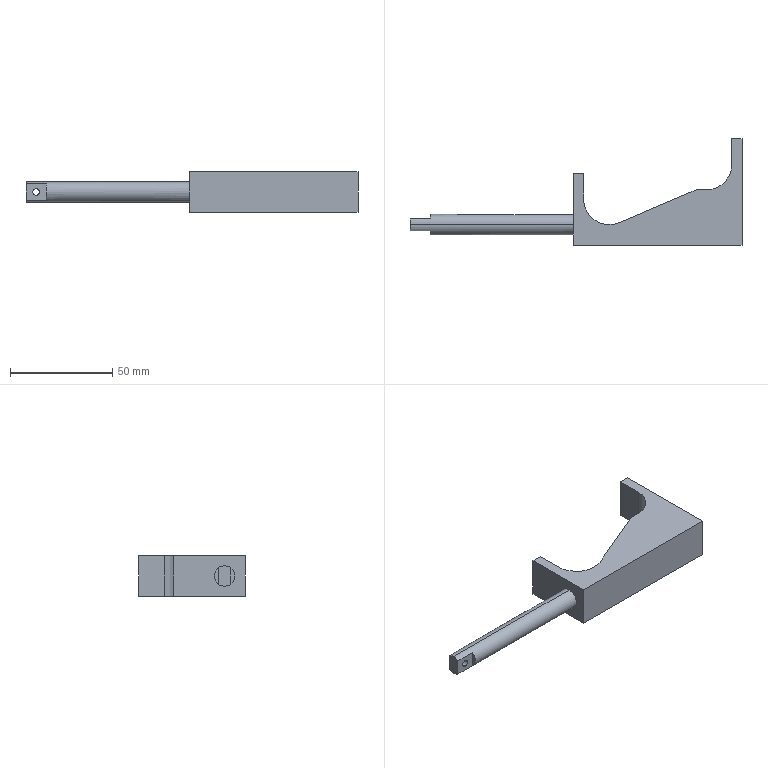Part | SolidWorks | features ICE 2, Extrusion 1, HoleWzd 1 | 1 solid | 22 faces | box 162.546 x 52 x 20 mm | volume 43317 mm3 | plane 16 | cylinder 6 | commonest cylinder face diameters 3.3 x2 10 x2 25 x2
STEP:
#1=CARTESIAN_POINT('',(-95.046,-3.,11.65));
#2=VERTEX_POINT('',#1);
#3=CARTESIAN_POINT('',(-95.046,-3.,8.35));
#4=VERTEX_POINT('',#3);
#5=CARTESIAN_POINT('',(-95.046,-3.,10.));
#6=DIRECTION('',(0.,-1.,0.));
#7=DIRECTION('',(0.,0.,-1.));
#8=AXIS2_PLACEMENT_3D('',#5,#6,#7);
#9=CIRCLE('',#8,1.65);
#10=EDGE_CURVE('',#2,#4,#9,.T.);
#11=ORIENTED_EDGE('',*,*,#10,.T.);
#12=CARTESIAN_POINT('',(-95.046,3.,8.35));
#13=VERTEX_POINT('',#12);
#14=CARTESIAN_POINT('',(-95.046,3.,8.35));
#15=DIRECTION('',(0.,1.,0.));
#16=VECTOR('',#15,1000.);
#17=LINE('',#14,#16);
#18=EDGE_CURVE('',#4,#13,#17,.T.);
#19=ORIENTED_EDGE('',*,*,#18,.T.);
#20=CARTESIAN_POINT('',(-95.046,3.,11.65));
#21=VERTEX_POINT('',#20);
#22=CARTESIAN_POINT('',(-95.046,3.,10.));
#23=DIRECTION('',(0.,1.,0.));
#24=DIRECTION('',(0.,0.,1.));
#25=AXIS2_PLACEMENT_3D('',#22,#23,#24);
#26=CIRCLE('',#25,1.65);
#27=EDGE_CURVE('',#13,#21,#26,.T.);
#28=ORIENTED_EDGE('',*,*,#27,.T.);
#29=CARTESIAN_POINT('',(-95.046,3.,11.65));
#30=DIRECTION('',(0.,1.,0.));
#31=VECTOR('',#30,1000.);
#32=LINE('',#29,#31);
#33=EDGE_CURVE('',#2,#21,#32,.T.);
#34=ORIENTED_EDGE('',*,*,#33,.F.);
#35=EDGE_LOOP('',(#11,#19,#28,#34));
#36=FACE_OUTER_BOUND('',#35,.T.);
#37=CARTESIAN_POINT('',(-95.046,3.,10.));
#38=DIRECTION('',(0.,1.,0.));
#39=DIRECTION('',(0.,0.,1.));
#40=AXIS2_PLACEMENT_3D('',#37,#38,#39);
#41=CYLINDRICAL_SURFACE('',#40,1.65);
#42=ADVANCED_FACE('',(#36),#41,.F.);
#43=CARTESIAN_POINT('',(-100.046,0.,15.));
#44=VERTEX_POINT('',#43);
#45=CARTESIAN_POINT('',(-100.046,3.,14.));
#46=VERTEX_POINT('',#45);
#47=CARTESIAN_POINT('',(-100.046,0.,10.));
#48=DIRECTION('',(-1.,0.,0.));
#49=DIRECTION('',(0.,0.,1.));
#50=AXIS2_PLACEMENT_3D('',#47,#48,#49);
#51=CIRCLE('',#50,5.);
#52=EDGE_CURVE('',#44,#46,#51,.T.);
#53=ORIENTED_EDGE('',*,*,#52,.F.);
#54=CARTESIAN_POINT('',(-20.046,0.,15.));
#55=VERTEX_POINT('',#54);
#56=CARTESIAN_POINT('',(-100.046,0.,15.));
#57=DIRECTION('',(1.,0.,0.));
#58=VECTOR('',#57,1000.);
#59=LINE('',#56,#58);
#60=EDGE_CURVE('',#44,#55,#59,.T.);
#61=ORIENTED_EDGE('',*,*,#60,.T.);
#62=CARTESIAN_POINT('',(-20.046,0.,5.));
#63=VERTEX_POINT('',#62);
#64=CARTESIAN_POINT('',(-20.046,0.,10.));
#65=DIRECTION('',(-1.,0.,0.));
#66=DIRECTION('',(0.,0.,-1.));
#67=AXIS2_PLACEMENT_3D('',#64,#65,#66);
#68=CIRCLE('',#67,5.);
#69=EDGE_CURVE('',#55,#63,#68,.T.);
#70=ORIENTED_EDGE('',*,*,#69,.T.);
#71=CARTESIAN_POINT('',(-100.046,0.,5.));
#72=VERTEX_POINT('',#71);
#73=CARTESIAN_POINT('',(-100.046,0.,5.));
#74=DIRECTION('',(1.,0.,0.));
#75=VECTOR('',#74,1000.);
#76=LINE('',#73,#75);
#77=EDGE_CURVE('',#72,#63,#76,.T.);
#78=ORIENTED_EDGE('',*,*,#77,.F.);
#79=CARTESIAN_POINT('',(-100.046,3.,6.));
#80=VERTEX_POINT('',#79);
#81=CARTESIAN_POINT('',(-100.046,0.,10.));
#82=DIRECTION('',(-1.,0.,0.));
#83=DIRECTION('',(0.,0.,1.));
#84=AXIS2_PLACEMENT_3D('',#81,#82,#83);
#85=CIRCLE('',#84,5.);
#86=EDGE_CURVE('',#80,#72,#85,.T.);
#87=ORIENTED_EDGE('',*,*,#86,.F.);
#88=CARTESIAN_POINT('',(-90.046,3.,6.));
#89=VERTEX_POINT('',#88);
#90=CARTESIAN_POINT('',(-100.046,3.,6.));
#91=DIRECTION('',(-1.,0.,0.));
#92=VECTOR('',#91,1000.);
#93=LINE('',#90,#92);
#94=EDGE_CURVE('',#89,#80,#93,.T.);
#95=ORIENTED_EDGE('',*,*,#94,.F.);
#96=CARTESIAN_POINT('',(-90.046,3.,14.));
#97=VERTEX_POINT('',#96);
#98=CARTESIAN_POINT('',(-90.046,0.,10.));
#99=DIRECTION('',(-1.,0.,0.));
#100=DIRECTION('',(0.,0.,1.));
#101=AXIS2_PLACEMENT_3D('',#98,#99,#100);
#102=CIRCLE('',#101,5.);
#103=EDGE_CURVE('',#97,#89,#102,.T.);
#104=ORIENTED_EDGE('',*,*,#103,.F.);
#105=CARTESIAN_POINT('',(-100.046,3.,14.));
#106=DIRECTION('',(1.,0.,0.));
#107=VECTOR('',#106,1000.);
#108=LINE('',#105,#107);
#109=EDGE_CURVE('',#46,#97,#108,.T.);
#110=ORIENTED_EDGE('',*,*,#109,.F.);
#111=EDGE_LOOP('',(#53,#61,#70,#78,#87,#95,#104,#110));
#112=FACE_OUTER_BOUND('',#111,.T.);
#113=CARTESIAN_POINT('',(-100.046,0.,10.));
#114=DIRECTION('',(1.,0.,0.));
#115=DIRECTION('',(0.,0.,-1.));
#116=AXIS2_PLACEMENT_3D('',#113,#114,#115);
#117=CYLINDRICAL_SURFACE('',#116,5.);
#118=ADVANCED_FACE('',(#112),#117,.T.);
#119=ORIENTED_EDGE('',*,*,#60,.F.);
#120=CARTESIAN_POINT('',(-100.046,-3.,14.));
#121=VERTEX_POINT('',#120);
#122=CARTESIAN_POINT('',(-100.046,0.,10.));
#123=DIRECTION('',(-1.,0.,0.));
#124=DIRECTION('',(0.,0.,1.));
#125=AXIS2_PLACEMENT_3D('',#122,#123,#124);
#126=CIRCLE('',#125,5.);
#127=EDGE_CURVE('',#121,#44,#126,.T.);
#128=ORIENTED_EDGE('',*,*,#127,.F.);
#129=CARTESIAN_POINT('',(-90.046,-3.,14.));
#130=VERTEX_POINT('',#129);
#131=CARTESIAN_POINT('',(-100.046,-3.,14.));
#132=DIRECTION('',(-1.,0.,0.));
#133=VECTOR('',#132,1000.);
#134=LINE('',#131,#133);
#135=EDGE_CURVE('',#130,#121,#134,.T.);
#136=ORIENTED_EDGE('',*,*,#135,.F.);
#137=CARTESIAN_POINT('',(-90.046,-3.,6.));
#138=VERTEX_POINT('',#137);
#139=CARTESIAN_POINT('',(-90.046,0.,10.));
#140=DIRECTION('',(-1.,0.,0.));
#141=DIRECTION('',(0.,0.,1.));
#142=AXIS2_PLACEMENT_3D('',#139,#140,#141);
#143=CIRCLE('',#142,5.);
#144=EDGE_CURVE('',#138,#130,#143,.T.);
#145=ORIENTED_EDGE('',*,*,#144,.F.);
#146=CARTESIAN_POINT('',(-100.046,-3.,6.));
#147=VERTEX_POINT('',#146);
#148=CARTESIAN_POINT('',(-100.046,-3.,6.));
#149=DIRECTION('',(1.,0.,0.));
#150=VECTOR('',#149,1000.);
#151=LINE('',#148,#150);
#152=EDGE_CURVE('',#147,#138,#151,.T.);
#153=ORIENTED_EDGE('',*,*,#152,.F.);
#154=CARTESIAN_POINT('',(-100.046,0.,10.));
#155=DIRECTION('',(-1.,0.,0.));
#156=DIRECTION('',(0.,0.,1.));
#157=AXIS2_PLACEMENT_3D('',#154,#155,#156);
#158=CIRCLE('',#157,5.);
#159=EDGE_CURVE('',#72,#147,#158,.T.);
#160=ORIENTED_EDGE('',*,*,#159,.F.);
#161=ORIENTED_EDGE('',*,*,#77,.T.);
#162=CARTESIAN_POINT('',(-20.046,0.,10.));
#163=DIRECTION('',(-1.,0.,0.));
#164=DIRECTION('',(0.,0.,-1.));
#165=AXIS2_PLACEMENT_3D('',#162,#163,#164);
#166=CIRCLE('',#165,5.);
#167=EDGE_CURVE('',#63,#55,#166,.T.);
#168=ORIENTED_EDGE('',*,*,#167,.T.);
#169=EDGE_LOOP('',(#119,#128,#136,#145,#153,#160,#161,#168));
#170=FACE_OUTER_BOUND('',#169,.T.);
#171=CARTESIAN_POINT('',(-100.046,0.,10.));
#172=DIRECTION('',(1.,0.,0.));
#173=DIRECTION('',(0.,0.,-1.));
#174=AXIS2_PLACEMENT_3D('',#171,#172,#173);
#175=CYLINDRICAL_SURFACE('',#174,5.);
#176=ADVANCED_FACE('',(#170),#175,.T.);
#177=ORIENTED_EDGE('',*,*,#127,.T.);
#178=ORIENTED_EDGE('',*,*,#52,.T.);
#179=CARTESIAN_POINT('',(-100.046,3.,10.));
#180=DIRECTION('',(0.,0.,-1.));
#181=VECTOR('',#180,1000.);
#182=LINE('',#179,#181);
#183=EDGE_CURVE('',#46,#80,#182,.T.);
#184=ORIENTED_EDGE('',*,*,#183,.T.);
#185=ORIENTED_EDGE('',*,*,#86,.T.);
#186=ORIENTED_EDGE('',*,*,#159,.T.);
#187=CARTESIAN_POINT('',(-100.046,-3.,10.));
#188=DIRECTION('',(0.,0.,1.));
#189=VECTOR('',#188,1000.);
#190=LINE('',#187,#189);
#191=EDGE_CURVE('',#147,#121,#190,.T.);
#192=ORIENTED_EDGE('',*,*,#191,.T.);
#193=EDGE_LOOP('',(#177,#178,#184,#185,#186,#192));
#194=FACE_OUTER_BOUND('',#193,.T.);
#195=CARTESIAN_POINT('',(-100.046,0.,10.));
#196=DIRECTION('',(-1.,0.,0.));
#197=DIRECTION('',(0.,0.,1.));
#198=AXIS2_PLACEMENT_3D('',#195,#196,#197);
#199=PLANE('',#198);
#200=ADVANCED_FACE('',(#194),#199,.T.);
#201=CARTESIAN_POINT('',(-20.046,25.,0.));
#202=VERTEX_POINT('',#201);
#203=CARTESIAN_POINT('',(-20.046,-10.,0.));
#204=VERTEX_POINT('',#203);
#205=CARTESIAN_POINT('',(-20.046,0.,0.));
#206=DIRECTION('',(0.,-1.,0.));
#207=VECTOR('',#206,1000.);
#208=LINE('',#205,#207);
#209=EDGE_CURVE('',#202,#204,#208,.T.);
#210=ORIENTED_EDGE('',*,*,#209,.T.);
#211=CARTESIAN_POINT('',(-20.046,-10.,20.));
#212=VERTEX_POINT('',#211);
#213=CARTESIAN_POINT('',(-20.046,-10.,20.));
#214=DIRECTION('',(0.,0.,-1.));
#215=VECTOR('',#214,1000.);
#216=LINE('',#213,#215);
#217=EDGE_CURVE('',#212,#204,#216,.T.);
#218=ORIENTED_EDGE('',*,*,#217,.F.);
#219=CARTESIAN_POINT('',(-20.046,25.,20.));
#220=VERTEX_POINT('',#219);
#221=CARTESIAN_POINT('',(-20.046,25.,20.));
#222=DIRECTION('',(0.,-1.,0.));
#223=VECTOR('',#222,1000.);
#224=LINE('',#221,#223);
#225=EDGE_CURVE('',#220,#212,#224,.T.);
#226=ORIENTED_EDGE('',*,*,#225,.F.);
#227=CARTESIAN_POINT('',(-20.046,25.,20.));
#228=DIRECTION('',(0.,0.,-1.));
#229=VECTOR('',#228,1000.);
#230=LINE('',#227,#229);
#231=EDGE_CURVE('',#220,#202,#230,.T.);
#232=ORIENTED_EDGE('',*,*,#231,.T.);
#233=EDGE_LOOP('',(#210,#218,#226,#232));
#234=FACE_OUTER_BOUND('',#233,.T.);
#235=ORIENTED_EDGE('',*,*,#167,.F.);
#236=ORIENTED_EDGE('',*,*,#69,.F.);
#237=EDGE_LOOP('',(#235,#236));
#238=FACE_BOUND('',#237,.T.);
#239=CARTESIAN_POINT('',(-20.046,0.,20.));
#240=DIRECTION('',(1.,0.,0.));
#241=DIRECTION('',(0.,0.,-1.));
#242=AXIS2_PLACEMENT_3D('',#239,#240,#241);
#243=PLANE('',#242);
#244=ADVANCED_FACE('',(#234,#238),#243,.F.);
#245=CARTESIAN_POINT('',(45.,17.,0.));
#246=VERTEX_POINT('',#245);
#247=CARTESIAN_POINT('',(40.,17.,0.));
#248=VERTEX_POINT('',#247);
#249=CARTESIAN_POINT('',(40.,17.,0.));
#250=DIRECTION('',(-1.,0.,0.));
#251=VECTOR('',#250,1000.);
#252=LINE('',#249,#251);
#253=EDGE_CURVE('',#246,#248,#252,.T.);
#254=ORIENTED_EDGE('',*,*,#253,.T.);
#255=CARTESIAN_POINT('',(40.,17.,20.));
#256=VERTEX_POINT('',#255);
#257=CARTESIAN_POINT('',(40.,17.,20.));
#258=DIRECTION('',(0.,0.,-1.));
#259=VECTOR('',#258,1000.);
#260=LINE('',#257,#259);
#261=EDGE_CURVE('',#256,#248,#260,.T.);
#262=ORIENTED_EDGE('',*,*,#261,.F.);
#263=CARTESIAN_POINT('',(45.,17.,20.));
#264=VERTEX_POINT('',#263);
#265=CARTESIAN_POINT('',(40.,17.,20.));
#266=DIRECTION('',(-1.,0.,0.));
#267=VECTOR('',#266,1000.);
#268=LINE('',#265,#267);
#269=EDGE_CURVE('',#264,#256,#268,.T.);
#270=ORIENTED_EDGE('',*,*,#269,.F.);
#271=CARTESIAN_POINT('',(45.,17.,20.));
#272=DIRECTION('',(0.,0.,-1.));
#273=VECTOR('',#272,1000.);
#274=LINE('',#271,#273);
#275=EDGE_CURVE('',#264,#246,#274,.T.);
#276=ORIENTED_EDGE('',*,*,#275,.T.);
#277=EDGE_LOOP('',(#254,#262,#270,#276));
#278=FACE_OUTER_BOUND('',#277,.T.);
#279=CARTESIAN_POINT('',(40.,17.,20.));
#280=DIRECTION('',(0.,-1.,0.));
#281=DIRECTION('',(1.,0.,0.));
#282=AXIS2_PLACEMENT_3D('',#279,#280,#281);
#283=PLANE('',#282);
#284=ADVANCED_FACE('',(#278),#283,.F.);
#285=CARTESIAN_POINT('',(2.343,0.9959,0.));
#286=VERTEX_POINT('',#285);
#287=CARTESIAN_POINT('',(2.343,0.9959,0.));
#288=DIRECTION('',(-0.9203,-0.3911,0.));
#289=VECTOR('',#288,1000.);
#290=LINE('',#287,#289);
#291=EDGE_CURVE('',#248,#286,#290,.T.);
#292=ORIENTED_EDGE('',*,*,#291,.T.);
#293=CARTESIAN_POINT('',(2.343,0.9959,20.));
#294=VERTEX_POINT('',#293);
#295=CARTESIAN_POINT('',(2.343,0.9959,20.));
#296=DIRECTION('',(0.,0.,-1.));
#297=VECTOR('',#296,1000.);
#298=LINE('',#295,#297);
#299=EDGE_CURVE('',#294,#286,#298,.T.);
#300=ORIENTED_EDGE('',*,*,#299,.F.);
#301=CARTESIAN_POINT('',(2.343,0.9959,20.));
#302=DIRECTION('',(-0.9203,-0.3911,0.));
#303=VECTOR('',#302,1000.);
#304=LINE('',#301,#303);
#305=EDGE_CURVE('',#256,#294,#304,.T.);
#306=ORIENTED_EDGE('',*,*,#305,.F.);
#307=ORIENTED_EDGE('',*,*,#261,.T.);
#308=EDGE_LOOP('',(#292,#300,#306,#307));
#309=FACE_OUTER_BOUND('',#308,.T.);
#310=CARTESIAN_POINT('',(2.343,0.9959,20.));
#311=DIRECTION('',(0.3911,-0.9203,0.));
#312=DIRECTION('',(0.9203,0.3911,0.));
#313=AXIS2_PLACEMENT_3D('',#310,#311,#312);
#314=PLANE('',#313);
#315=ADVANCED_FACE('',(#309),#314,.F.);
#316=CARTESIAN_POINT('',(-15.046,12.5,0.));
#317=VERTEX_POINT('',#316);
#318=CARTESIAN_POINT('',(-2.546,12.5,0.));
#319=DIRECTION('',(0.,0.,-1.));
#320=DIRECTION('',(1.,0.,0.));
#321=AXIS2_PLACEMENT_3D('',#318,#319,#320);
#322=CIRCLE('',#321,12.5);
#323=EDGE_CURVE('',#286,#317,#322,.T.);
#324=ORIENTED_EDGE('',*,*,#323,.T.);
#325=CARTESIAN_POINT('',(-15.046,12.5,20.));
#326=VERTEX_POINT('',#325);
#327=CARTESIAN_POINT('',(-15.046,12.5,20.));
#328=DIRECTION('',(0.,0.,-1.));
#329=VECTOR('',#328,1000.);
#330=LINE('',#327,#329);
#331=EDGE_CURVE('',#326,#317,#330,.T.);
#332=ORIENTED_EDGE('',*,*,#331,.F.);
#333=CARTESIAN_POINT('',(-2.546,12.5,20.));
#334=DIRECTION('',(0.,0.,-1.));
#335=DIRECTION('',(1.,0.,0.));
#336=AXIS2_PLACEMENT_3D('',#333,#334,#335);
#337=CIRCLE('',#336,12.5);
#338=EDGE_CURVE('',#294,#326,#337,.T.);
#339=ORIENTED_EDGE('',*,*,#338,.F.);
#340=ORIENTED_EDGE('',*,*,#299,.T.);
#341=EDGE_LOOP('',(#324,#332,#339,#340));
#342=FACE_OUTER_BOUND('',#341,.T.);
#343=CARTESIAN_POINT('',(-2.546,12.5,20.));
#344=DIRECTION('',(0.,0.,-1.));
#345=DIRECTION('',(-1.,0.,0.));
#346=AXIS2_PLACEMENT_3D('',#343,#344,#345);
#347=CYLINDRICAL_SURFACE('',#346,12.5);
#348=ADVANCED_FACE('',(#342),#347,.F.);
#349=CARTESIAN_POINT('',(-15.046,25.,0.));
#350=VERTEX_POINT('',#349);
#351=CARTESIAN_POINT('',(-15.046,12.5,0.));
#352=DIRECTION('',(0.,1.,0.));
#353=VECTOR('',#352,1000.);
#354=LINE('',#351,#353);
#355=EDGE_CURVE('',#317,#350,#354,.T.);
#356=ORIENTED_EDGE('',*,*,#355,.T.);
#357=CARTESIAN_POINT('',(-15.046,25.,20.));
#358=VERTEX_POINT('',#357);
#359=CARTESIAN_POINT('',(-15.046,25.,20.));
#360=DIRECTION('',(0.,0.,-1.));
#361=VECTOR('',#360,1000.);
#362=LINE('',#359,#361);
#363=EDGE_CURVE('',#358,#350,#362,.T.);
#364=ORIENTED_EDGE('',*,*,#363,.F.);
#365=CARTESIAN_POINT('',(-15.046,12.5,20.));
#366=DIRECTION('',(0.,1.,0.));
#367=VECTOR('',#366,1000.);
#368=LINE('',#365,#367);
#369=EDGE_CURVE('',#326,#358,#368,.T.);
#370=ORIENTED_EDGE('',*,*,#369,.F.);
#371=ORIENTED_EDGE('',*,*,#331,.T.);
#372=EDGE_LOOP('',(#356,#364,#370,#371));
#373=FACE_OUTER_BOUND('',#372,.T.);
#374=CARTESIAN_POINT('',(-15.046,12.5,20.));
#375=DIRECTION('',(-1.,0.,0.));
#376=DIRECTION('',(0.,0.,1.));
#377=AXIS2_PLACEMENT_3D('',#374,#375,#376);
#378=PLANE('',#377);
#379=ADVANCED_FACE('',(#373),#378,.F.);
#380=CARTESIAN_POINT('',(-15.046,25.,0.));
#381=DIRECTION('',(-1.,0.,0.));
#382=VECTOR('',#381,1000.);
#383=LINE('',#380,#382);
#384=EDGE_CURVE('',#350,#202,#383,.T.);
#385=ORIENTED_EDGE('',*,*,#384,.T.);
#386=ORIENTED_EDGE('',*,*,#231,.F.);
#387=CARTESIAN_POINT('',(-15.046,25.,20.));
#388=DIRECTION('',(-1.,0.,0.));
#389=VECTOR('',#388,1000.);
#390=LINE('',#387,#389);
#391=EDGE_CURVE('',#358,#220,#390,.T.);
#392=ORIENTED_EDGE('',*,*,#391,.F.);
#393=ORIENTED_EDGE('',*,*,#363,.T.);
#394=EDGE_LOOP('',(#385,#386,#392,#393));
#395=FACE_OUTER_BOUND('',#394,.T.);
#396=CARTESIAN_POINT('',(-15.046,25.,20.));
#397=DIRECTION('',(0.,-1.,0.));
#398=DIRECTION('',(0.,0.,-1.));
#399=AXIS2_PLACEMENT_3D('',#396,#397,#398);
#400=PLANE('',#399);
#401=ADVANCED_FACE('',(#395),#400,.F.);
#402=CARTESIAN_POINT('',(62.5,-10.,0.));
#403=VERTEX_POINT('',#402);
#404=CARTESIAN_POINT('',(57.5,-10.,0.));
#405=DIRECTION('',(1.,0.,0.));
#406=VECTOR('',#405,1000.);
#407=LINE('',#404,#406);
#408=EDGE_CURVE('',#204,#403,#407,.T.);
#409=ORIENTED_EDGE('',*,*,#408,.T.);
#410=CARTESIAN_POINT('',(62.5,-10.,20.));
#411=VERTEX_POINT('',#410);
#412=CARTESIAN_POINT('',(62.5,-10.,20.));
#413=DIRECTION('',(0.,0.,-1.));
#414=VECTOR('',#413,1000.);
#415=LINE('',#412,#414);
#416=EDGE_CURVE('',#411,#403,#415,.T.);
#417=ORIENTED_EDGE('',*,*,#416,.F.);
#418=CARTESIAN_POINT('',(-20.046,-10.,20.));
#419=DIRECTION('',(1.,0.,0.));
#420=VECTOR('',#419,1000.);
#421=LINE('',#418,#420);
#422=EDGE_CURVE('',#212,#411,#421,.T.);
#423=ORIENTED_EDGE('',*,*,#422,.F.);
#424=ORIENTED_EDGE('',*,*,#217,.T.);
#425=EDGE_LOOP('',(#409,#417,#423,#424));
#426=FACE_OUTER_BOUND('',#425,.T.);
#427=CARTESIAN_POINT('',(57.5,-10.,20.));
#428=DIRECTION('',(0.,1.,0.));
#429=DIRECTION('',(0.,0.,1.));
#430=AXIS2_PLACEMENT_3D('',#427,#428,#429);
#431=PLANE('',#430);
#432=ADVANCED_FACE('',(#426),#431,.F.);
#433=CARTESIAN_POINT('',(62.5,42.,0.));
#434=VERTEX_POINT('',#433);
#435=CARTESIAN_POINT('',(62.5,-10.,0.));
#436=DIRECTION('',(0.,1.,0.));
#437=VECTOR('',#436,1000.);
#438=LINE('',#435,#437);
#439=EDGE_CURVE('',#403,#434,#438,.T.);
#440=ORIENTED_EDGE('',*,*,#439,.T.);
#441=CARTESIAN_POINT('',(62.5,42.,20.));
#442=VERTEX_POINT('',#441);
#443=CARTESIAN_POINT('',(62.5,42.,20.));
#444=DIRECTION('',(0.,0.,-1.));
#445=VECTOR('',#444,1000.);
#446=LINE('',#443,#445);
#447=EDGE_CURVE('',#442,#434,#446,.T.);
#448=ORIENTED_EDGE('',*,*,#447,.F.);
#449=CARTESIAN_POINT('',(62.5,-10.,20.));
#450=DIRECTION('',(0.,1.,0.));
#451=VECTOR('',#450,1000.);
#452=LINE('',#449,#451);
#453=EDGE_CURVE('',#411,#442,#452,.T.);
#454=ORIENTED_EDGE('',*,*,#453,.F.);
#455=ORIENTED_EDGE('',*,*,#416,.T.);
#456=EDGE_LOOP('',(#440,#448,#454,#455));
#457=FACE_OUTER_BOUND('',#456,.T.);
#458=CARTESIAN_POINT('',(62.5,-10.,20.));
#459=DIRECTION('',(-1.,0.,0.));
#460=DIRECTION('',(0.,0.,1.));
#461=AXIS2_PLACEMENT_3D('',#458,#459,#460);
#462=PLANE('',#461);
#463=ADVANCED_FACE('',(#457),#462,.F.);
#464=CARTESIAN_POINT('',(57.5,42.,0.));
#465=VERTEX_POINT('',#464);
#466=CARTESIAN_POINT('',(62.5,42.,0.));
#467=DIRECTION('',(-1.,0.,0.));
#468=VECTOR('',#467,1000.);
#469=LINE('',#466,#468);
#470=EDGE_CURVE('',#434,#465,#469,.T.);
#471=ORIENTED_EDGE('',*,*,#470,.T.);
#472=CARTESIAN_POINT('',(57.5,42.,20.));
#473=VERTEX_POINT('',#472);
#474=CARTESIAN_POINT('',(57.5,42.,20.));
#475=DIRECTION('',(0.,0.,-1.));
#476=VECTOR('',#475,1000.);
#477=LINE('',#474,#476);
#478=EDGE_CURVE('',#473,#465,#477,.T.);
#479=ORIENTED_EDGE('',*,*,#478,.F.);
#480=CARTESIAN_POINT('',(62.5,42.,20.));
#481=DIRECTION('',(-1.,0.,0.));
#482=VECTOR('',#481,1000.);
#483=LINE('',#480,#482);
#484=EDGE_CURVE('',#442,#473,#483,.T.);
#485=ORIENTED_EDGE('',*,*,#484,.F.);
#486=ORIENTED_EDGE('',*,*,#447,.T.);
#487=EDGE_LOOP('',(#471,#479,#485,#486));
#488=FACE_OUTER_BOUND('',#487,.T.);
#489=CARTESIAN_POINT('',(62.5,42.,20.));
#490=DIRECTION('',(0.,-1.,0.));
#491=DIRECTION('',(0.,0.,-1.));
#492=AXIS2_PLACEMENT_3D('',#489,#490,#491);
#493=PLANE('',#492);
#494=ADVANCED_FACE('',(#488),#493,.F.);
#495=CARTESIAN_POINT('',(57.5,29.5,0.));
#496=VERTEX_POINT('',#495);
#497=CARTESIAN_POINT('',(57.5,42.,0.));
#498=DIRECTION('',(0.,-1.,0.));
#499=VECTOR('',#498,1000.);
#500=LINE('',#497,#499);
#501=EDGE_CURVE('',#465,#496,#500,.T.);
#502=ORIENTED_EDGE('',*,*,#501,.T.);
#503=CARTESIAN_POINT('',(57.5,29.5,20.));
#504=VERTEX_POINT('',#503);
#505=CARTESIAN_POINT('',(57.5,29.5,20.));
#506=DIRECTION('',(0.,0.,-1.));
#507=VECTOR('',#506,1000.);
#508=LINE('',#505,#507);
#509=EDGE_CURVE('',#504,#496,#508,.T.);
#510=ORIENTED_EDGE('',*,*,#509,.F.);
#511=CARTESIAN_POINT('',(57.5,42.,20.));
#512=DIRECTION('',(0.,-1.,0.));
#513=VECTOR('',#512,1000.);
#514=LINE('',#511,#513);
#515=EDGE_CURVE('',#473,#504,#514,.T.);
#516=ORIENTED_EDGE('',*,*,#515,.F.);
#517=ORIENTED_EDGE('',*,*,#478,.T.);
#518=EDGE_LOOP('',(#502,#510,#516,#517));
#519=FACE_OUTER_BOUND('',#518,.T.);
#520=CARTESIAN_POINT('',(57.5,42.,20.));
#521=DIRECTION('',(1.,0.,0.));
#522=DIRECTION('',(0.,0.,-1.));
#523=AXIS2_PLACEMENT_3D('',#520,#521,#522);
#524=PLANE('',#523);
#525=ADVANCED_FACE('',(#519),#524,.F.);
#526=CARTESIAN_POINT('',(45.,29.5,0.));
#527=DIRECTION('',(0.,0.,-1.));
#528=DIRECTION('',(1.,0.,0.));
#529=AXIS2_PLACEMENT_3D('',#526,#527,#528);
#530=CIRCLE('',#529,12.5);
#531=EDGE_CURVE('',#496,#246,#530,.T.);
#532=ORIENTED_EDGE('',*,*,#531,.T.);
#533=ORIENTED_EDGE('',*,*,#275,.F.);
#534=CARTESIAN_POINT('',(45.,29.5,20.));
#535=DIRECTION('',(0.,0.,-1.));
#536=DIRECTION('',(1.,0.,0.));
#537=AXIS2_PLACEMENT_3D('',#534,#535,#536);
#538=CIRCLE('',#537,12.5);
#539=EDGE_CURVE('',#504,#264,#538,.T.);
#540=ORIENTED_EDGE('',*,*,#539,.F.);
#541=ORIENTED_EDGE('',*,*,#509,.T.);
#542=EDGE_LOOP('',(#532,#533,#540,#541));
#543=FACE_OUTER_BOUND('',#542,.T.);
#544=CARTESIAN_POINT('',(45.,29.5,20.));
#545=DIRECTION('',(0.,0.,-1.));
#546=DIRECTION('',(-1.,0.,0.));
#547=AXIS2_PLACEMENT_3D('',#544,#545,#546);
#548=CYLINDRICAL_SURFACE('',#547,12.5);
#549=ADVANCED_FACE('',(#543),#548,.F.);
#550=ORIENTED_EDGE('',*,*,#269,.T.);
#551=ORIENTED_EDGE('',*,*,#305,.T.);
#552=ORIENTED_EDGE('',*,*,#338,.T.);
#553=ORIENTED_EDGE('',*,*,#369,.T.);
#554=ORIENTED_EDGE('',*,*,#391,.T.);
#555=ORIENTED_EDGE('',*,*,#225,.T.);
#556=ORIENTED_EDGE('',*,*,#422,.T.);
#557=ORIENTED_EDGE('',*,*,#453,.T.);
#558=ORIENTED_EDGE('',*,*,#484,.T.);
#559=ORIENTED_EDGE('',*,*,#515,.T.);
#560=ORIENTED_EDGE('',*,*,#539,.T.);
#561=EDGE_LOOP('',(#550,#551,#552,#553,#554,#555,#556,#557,#558,#559,#560));
#562=FACE_OUTER_BOUND('',#561,.T.);
#563=CARTESIAN_POINT('',(45.,29.5,20.));
#564=DIRECTION('',(0.,0.,1.));
#565=DIRECTION('',(1.,0.,0.));
#566=AXIS2_PLACEMENT_3D('',#563,#564,#565);
#567=PLANE('',#566);
#568=ADVANCED_FACE('',(#562),#567,.T.);
#569=ORIENTED_EDGE('',*,*,#253,.F.);
#570=ORIENTED_EDGE('',*,*,#531,.F.);
#571=ORIENTED_EDGE('',*,*,#501,.F.);
#572=ORIENTED_EDGE('',*,*,#470,.F.);
#573=ORIENTED_EDGE('',*,*,#439,.F.);
#574=ORIENTED_EDGE('',*,*,#408,.F.);
#575=ORIENTED_EDGE('',*,*,#209,.F.);
#576=ORIENTED_EDGE('',*,*,#384,.F.);
#577=ORIENTED_EDGE('',*,*,#355,.F.);
#578=ORIENTED_EDGE('',*,*,#323,.F.);
#579=ORIENTED_EDGE('',*,*,#291,.F.);
#580=EDGE_LOOP('',(#569,#570,#571,#572,#573,#574,#575,#576,#577,#578,#579));
#581=FACE_OUTER_BOUND('',#580,.T.);
#582=CARTESIAN_POINT('',(45.,29.5,0.));
#583=DIRECTION('',(0.,0.,1.));
#584=DIRECTION('',(1.,0.,0.));
#585=AXIS2_PLACEMENT_3D('',#582,#583,#584);
#586=PLANE('',#585);
#587=ADVANCED_FACE('',(#581),#586,.F.);
#588=ORIENTED_EDGE('',*,*,#10,.F.);
#589=CARTESIAN_POINT('',(-95.046,-3.,10.));
#590=DIRECTION('',(0.,-1.,0.));
#591=DIRECTION('',(0.,0.,-1.));
#592=AXIS2_PLACEMENT_3D('',#589,#590,#591);
#593=CIRCLE('',#592,1.65);
#594=EDGE_CURVE('',#4,#2,#593,.T.);
#595=ORIENTED_EDGE('',*,*,#594,.F.);
#596=EDGE_LOOP('',(#588,#595));
#597=FACE_BOUND('',#596,.T.);
#598=ORIENTED_EDGE('',*,*,#152,.T.);
#599=CARTESIAN_POINT('',(-90.046,-3.,3.784));
#600=DIRECTION('',(0.,0.,1.));
#601=VECTOR('',#600,1000.);
#602=LINE('',#599,#601);
#603=EDGE_CURVE('',#138,#130,#602,.T.);
#604=ORIENTED_EDGE('',*,*,#603,.T.);
#605=ORIENTED_EDGE('',*,*,#135,.T.);
#606=ORIENTED_EDGE('',*,*,#191,.F.);
#607=EDGE_LOOP('',(#598,#604,#605,#606));
#608=FACE_OUTER_BOUND('',#607,.T.);
#609=CARTESIAN_POINT('',(-90.046,-3.,3.784));
#610=DIRECTION('',(0.,-1.,0.));
#611=DIRECTION('',(0.,0.,-1.));
#612=AXIS2_PLACEMENT_3D('',#609,#610,#611);
#613=PLANE('',#612);
#614=ADVANCED_FACE('',(#597,#608),#613,.T.);
#615=ORIENTED_EDGE('',*,*,#144,.T.);
#616=ORIENTED_EDGE('',*,*,#603,.F.);
#617=EDGE_LOOP('',(#615,#616));
#618=FACE_OUTER_BOUND('',#617,.T.);
#619=CARTESIAN_POINT('',(-90.046,16.,10.));
#620=DIRECTION('',(-1.,0.,0.));
#621=DIRECTION('',(0.,0.,1.));
#622=AXIS2_PLACEMENT_3D('',#619,#620,#621);
#623=PLANE('',#622);
#624=ADVANCED_FACE('',(#618),#623,.T.);
#625=ORIENTED_EDGE('',*,*,#103,.T.);
#626=CARTESIAN_POINT('',(-90.046,3.,3.784));
#627=DIRECTION('',(0.,0.,-1.));
#628=VECTOR('',#627,1000.);
#629=LINE('',#626,#628);
#630=EDGE_CURVE('',#97,#89,#629,.T.);
#631=ORIENTED_EDGE('',*,*,#630,.F.);
#632=EDGE_LOOP('',(#625,#631));
#633=FACE_OUTER_BOUND('',#632,.T.);
#634=CARTESIAN_POINT('',(-90.046,16.,10.));
#635=DIRECTION('',(-1.,0.,0.));
#636=DIRECTION('',(0.,0.,1.));
#637=AXIS2_PLACEMENT_3D('',#634,#635,#636);
#638=PLANE('',#637);
#639=ADVANCED_FACE('',(#633),#638,.T.);
#640=CARTESIAN_POINT('',(-95.046,3.,10.));
#641=DIRECTION('',(0.,1.,0.));
#642=DIRECTION('',(0.,0.,1.));
#643=AXIS2_PLACEMENT_3D('',#640,#641,#642);
#644=CIRCLE('',#643,1.65);
#645=EDGE_CURVE('',#21,#13,#644,.T.);
#646=ORIENTED_EDGE('',*,*,#645,.F.);
#647=ORIENTED_EDGE('',*,*,#27,.F.);
#648=EDGE_LOOP('',(#646,#647));
#649=FACE_BOUND('',#648,.T.);
#650=ORIENTED_EDGE('',*,*,#109,.T.);
#651=ORIENTED_EDGE('',*,*,#630,.T.);
#652=ORIENTED_EDGE('',*,*,#94,.T.);
#653=ORIENTED_EDGE('',*,*,#183,.F.);
#654=EDGE_LOOP('',(#650,#651,#652,#653));
#655=FACE_OUTER_BOUND('',#654,.T.);
#656=CARTESIAN_POINT('',(-90.046,3.,3.784));
#657=DIRECTION('',(0.,1.,0.));
#658=DIRECTION('',(0.,0.,1.));
#659=AXIS2_PLACEMENT_3D('',#656,#657,#658);
#660=PLANE('',#659);
#661=ADVANCED_FACE('',(#649,#655),#660,.T.);
#662=ORIENTED_EDGE('',*,*,#18,.F.);
#663=ORIENTED_EDGE('',*,*,#594,.T.);
#664=ORIENTED_EDGE('',*,*,#33,.T.);
#665=ORIENTED_EDGE('',*,*,#645,.T.);
#666=EDGE_LOOP('',(#662,#663,#664,#665));
#667=FACE_OUTER_BOUND('',#666,.T.);
#668=CARTESIAN_POINT('',(-95.046,3.,10.));
#669=DIRECTION('',(0.,1.,0.));
#670=DIRECTION('',(0.,0.,1.));
#671=AXIS2_PLACEMENT_3D('',#668,#669,#670);
#672=CYLINDRICAL_SURFACE('',#671,1.65);
#673=ADVANCED_FACE('',(#667),#672,.F.);
#674=CLOSED_SHELL('',(#42,#118,#176,#200,#244,#284,#315,#348,#379,#401,#432,#463,#494,#525,#549,#568,#587,#614,#624,#639,#661,#673));
#675=MANIFOLD_SOLID_BREP('',#674);
#676=CARTESIAN_POINT('',(0.,0.,0.));
#677=DIRECTION('',(0.,0.,1.));
#678=DIRECTION('',(1.,0.,0.));
#679=AXIS2_PLACEMENT_3D('',#676,#677,#678);
#680=(LENGTH_UNIT()NAMED_UNIT(*)SI_UNIT(.MILLI.,.METRE.));
#681=UNCERTAINTY_MEASURE_WITH_UNIT(LENGTH_MEASURE(0.00001),#680,'','');
#682=(NAMED_UNIT(*)PLANE_ANGLE_UNIT()SI_UNIT($,.RADIAN.));
#683=(NAMED_UNIT(*)SI_UNIT($,.STERADIAN.)SOLID_ANGLE_UNIT());
#684=(GEOMETRIC_REPRESENTATION_CONTEXT(3)GLOBAL_UNCERTAINTY_ASSIGNED_CONTEXT((#681))GLOBAL_UNIT_ASSIGNED_CONTEXT((#680,#682,#683))REPRESENTATION_CONTEXT('',''));
#685=ADVANCED_BREP_SHAPE_REPRESENTATION('',(#675,#679),#684);